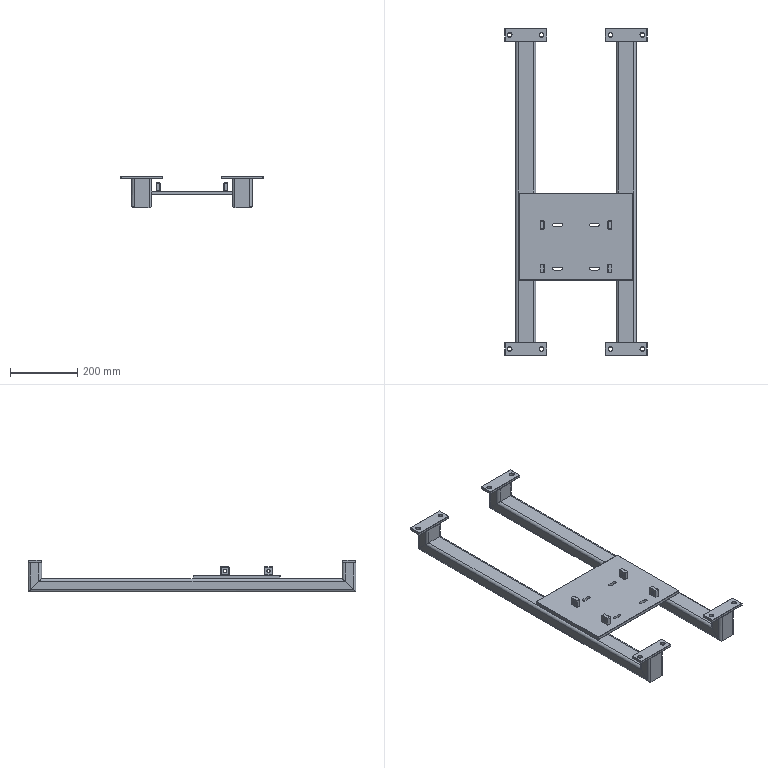Part | SolidWorks | 11 solids | 370 faces | box 425 x 976 x 95 mm | volume 2540191 mm3 | plane 230 | cylinder 92 | cone 48 | commonest cylinder face diameters 8 x24 16 x24 12 x16 9 x12 8.5 x8 10 x8